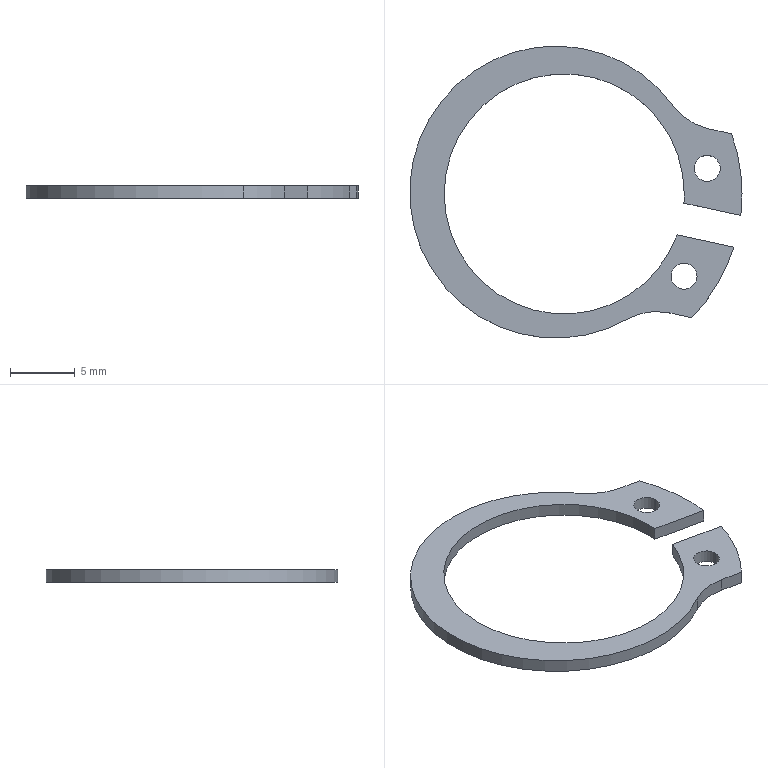Part | SolidWorks | features BaseBody 1 | 1 solid | 19 faces | box 25.605 x 22.5 x 1 mm | volume 159.858 mm3 | cylinder 13 | plane 6 | commonest cylinder face diameters 2 x4 18.5 x3 27.4 x3 9 x2 22.5 x1
STEP:
#1=CARTESIAN_POINT('',(-11.273,1593.906,-381.));
#2=VERTEX_POINT('',#1);
#3=CARTESIAN_POINT('',(-9.273,1593.906,-381.));
#4=VERTEX_POINT('',#3);
#5=CARTESIAN_POINT('',(-10.273,1593.906,-381.));
#6=DIRECTION('',(0.,0.,1.));
#7=DIRECTION('',(1.,0.,0.));
#8=AXIS2_PLACEMENT_3D('',#5,#6,#7);
#9=CIRCLE('',#8,1.);
#10=EDGE_CURVE('',#2,#4,#9,.T.);
#11=ORIENTED_EDGE('',*,*,#10,.F.);
#12=CARTESIAN_POINT('',(-11.273,1593.906,-380.));
#13=VERTEX_POINT('',#12);
#14=CARTESIAN_POINT('',(-11.273,1593.906,-381.));
#15=DIRECTION('',(0.,0.,1.));
#16=VECTOR('',#15,1000.);
#17=LINE('',#14,#16);
#18=EDGE_CURVE('',#2,#13,#17,.T.);
#19=ORIENTED_EDGE('',*,*,#18,.T.);
#20=CARTESIAN_POINT('',(-9.273,1593.906,-380.));
#21=VERTEX_POINT('',#20);
#22=CARTESIAN_POINT('',(-10.273,1593.906,-380.));
#23=DIRECTION('',(0.,0.,-1.));
#24=DIRECTION('',(1.,0.,0.));
#25=AXIS2_PLACEMENT_3D('',#22,#23,#24);
#26=CIRCLE('',#25,1.);
#27=EDGE_CURVE('',#21,#13,#26,.T.);
#28=ORIENTED_EDGE('',*,*,#27,.F.);
#29=CARTESIAN_POINT('',(-9.273,1593.906,-381.));
#30=DIRECTION('',(0.,0.,1.));
#31=VECTOR('',#30,1000.);
#32=LINE('',#29,#31);
#33=EDGE_CURVE('',#4,#21,#32,.T.);
#34=ORIENTED_EDGE('',*,*,#33,.F.);
#35=EDGE_LOOP('',(#11,#19,#28,#34));
#36=FACE_OUTER_BOUND('',#35,.T.);
#37=CARTESIAN_POINT('',(-10.273,1593.906,-381.));
#38=DIRECTION('',(0.,0.,1.));
#39=DIRECTION('',(1.,0.,0.));
#40=AXIS2_PLACEMENT_3D('',#37,#38,#39);
#41=CYLINDRICAL_SURFACE('',#40,1.);
#42=ADVANCED_FACE('',(#36),#41,.F.);
#43=CARTESIAN_POINT('',(-13.066,1585.597,-381.));
#44=VERTEX_POINT('',#43);
#45=CARTESIAN_POINT('',(-11.066,1585.597,-381.));
#46=VERTEX_POINT('',#45);
#47=CARTESIAN_POINT('',(-12.066,1585.597,-381.));
#48=DIRECTION('',(0.,0.,1.));
#49=DIRECTION('',(1.,0.,0.));
#50=AXIS2_PLACEMENT_3D('',#47,#48,#49);
#51=CIRCLE('',#50,1.);
#52=EDGE_CURVE('',#44,#46,#51,.T.);
#53=ORIENTED_EDGE('',*,*,#52,.F.);
#54=CARTESIAN_POINT('',(-13.066,1585.597,-380.));
#55=VERTEX_POINT('',#54);
#56=CARTESIAN_POINT('',(-13.066,1585.597,-381.));
#57=DIRECTION('',(0.,0.,1.));
#58=VECTOR('',#57,1000.);
#59=LINE('',#56,#58);
#60=EDGE_CURVE('',#44,#55,#59,.T.);
#61=ORIENTED_EDGE('',*,*,#60,.T.);
#62=CARTESIAN_POINT('',(-11.066,1585.597,-380.));
#63=VERTEX_POINT('',#62);
#64=CARTESIAN_POINT('',(-12.066,1585.597,-380.));
#65=DIRECTION('',(0.,0.,-1.));
#66=DIRECTION('',(1.,0.,0.));
#67=AXIS2_PLACEMENT_3D('',#64,#65,#66);
#68=CIRCLE('',#67,1.);
#69=EDGE_CURVE('',#63,#55,#68,.T.);
#70=ORIENTED_EDGE('',*,*,#69,.F.);
#71=CARTESIAN_POINT('',(-11.066,1585.597,-381.));
#72=DIRECTION('',(0.,0.,1.));
#73=VECTOR('',#72,1000.);
#74=LINE('',#71,#73);
#75=EDGE_CURVE('',#46,#63,#74,.T.);
#76=ORIENTED_EDGE('',*,*,#75,.F.);
#77=EDGE_LOOP('',(#53,#61,#70,#76));
#78=FACE_OUTER_BOUND('',#77,.T.);
#79=CARTESIAN_POINT('',(-12.066,1585.597,-381.));
#80=DIRECTION('',(0.,0.,1.));
#81=DIRECTION('',(1.,0.,0.));
#82=AXIS2_PLACEMENT_3D('',#79,#80,#81);
#83=CYLINDRICAL_SURFACE('',#82,1.);
#84=ADVANCED_FACE('',(#78),#83,.F.);
#85=CARTESIAN_POINT('',(-7.699,1590.281,-381.));
#86=VERTEX_POINT('',#85);
#87=CARTESIAN_POINT('',(-7.599,1591.937,-381.));
#88=VERTEX_POINT('',#87);
#89=CARTESIAN_POINT('',(-21.299,1591.937,-381.));
#90=DIRECTION('',(0.,0.,1.));
#91=DIRECTION('',(1.,0.,0.));
#92=AXIS2_PLACEMENT_3D('',#89,#90,#91);
#93=CIRCLE('',#92,13.7);
#94=EDGE_CURVE('',#86,#88,#93,.T.);
#95=ORIENTED_EDGE('',*,*,#94,.T.);
#96=CARTESIAN_POINT('',(-7.599,1591.937,-380.));
#97=VERTEX_POINT('',#96);
#98=CARTESIAN_POINT('',(-7.599,1591.937,-381.));
#99=DIRECTION('',(0.,0.,1.));
#100=VECTOR('',#99,1000.);
#101=LINE('',#98,#100);
#102=EDGE_CURVE('',#88,#97,#101,.T.);
#103=ORIENTED_EDGE('',*,*,#102,.T.);
#104=CARTESIAN_POINT('',(-7.699,1590.281,-380.));
#105=VERTEX_POINT('',#104);
#106=CARTESIAN_POINT('',(-21.299,1591.937,-380.));
#107=DIRECTION('',(0.,0.,1.));
#108=DIRECTION('',(1.,0.,0.));
#109=AXIS2_PLACEMENT_3D('',#106,#107,#108);
#110=CIRCLE('',#109,13.7);
#111=EDGE_CURVE('',#105,#97,#110,.T.);
#112=ORIENTED_EDGE('',*,*,#111,.F.);
#113=CARTESIAN_POINT('',(-7.699,1590.281,-381.));
#114=DIRECTION('',(0.,0.,-1.));
#115=VECTOR('',#114,1000.);
#116=LINE('',#113,#115);
#117=EDGE_CURVE('',#105,#86,#116,.T.);
#118=ORIENTED_EDGE('',*,*,#117,.T.);
#119=EDGE_LOOP('',(#95,#103,#112,#118));
#120=FACE_OUTER_BOUND('',#119,.T.);
#121=CARTESIAN_POINT('',(-21.299,1591.937,-381.));
#122=DIRECTION('',(0.,0.,1.));
#123=DIRECTION('',(1.,0.,0.));
#124=AXIS2_PLACEMENT_3D('',#121,#122,#123);
#125=CYLINDRICAL_SURFACE('',#124,13.7);
#126=ADVANCED_FACE('',(#120),#125,.T.);
#127=CARTESIAN_POINT('',(-30.549,1591.937,-381.));
#128=VERTEX_POINT('',#127);
#129=CARTESIAN_POINT('',(-12.603,1588.782,-381.));
#130=VERTEX_POINT('',#129);
#131=CARTESIAN_POINT('',(-21.299,1591.937,-381.));
#132=DIRECTION('',(0.,0.,1.));
#133=DIRECTION('',(1.,0.,0.));
#134=AXIS2_PLACEMENT_3D('',#131,#132,#133);
#135=CIRCLE('',#134,9.25);
#136=EDGE_CURVE('',#128,#130,#135,.T.);
#137=ORIENTED_EDGE('',*,*,#136,.F.);
#138=CARTESIAN_POINT('',(-30.549,1591.937,-380.));
#139=VERTEX_POINT('',#138);
#140=CARTESIAN_POINT('',(-30.549,1591.937,-381.));
#141=DIRECTION('',(0.,0.,1.));
#142=VECTOR('',#141,1000.);
#143=LINE('',#140,#142);
#144=EDGE_CURVE('',#128,#139,#143,.T.);
#145=ORIENTED_EDGE('',*,*,#144,.T.);
#146=CARTESIAN_POINT('',(-12.603,1588.782,-380.));
#147=VERTEX_POINT('',#146);
#148=CARTESIAN_POINT('',(-21.299,1591.937,-380.));
#149=DIRECTION('',(0.,0.,-1.));
#150=DIRECTION('',(1.,0.,0.));
#151=AXIS2_PLACEMENT_3D('',#148,#149,#150);
#152=CIRCLE('',#151,9.25);
#153=EDGE_CURVE('',#147,#139,#152,.T.);
#154=ORIENTED_EDGE('',*,*,#153,.F.);
#155=CARTESIAN_POINT('',(-12.603,1588.782,-381.));
#156=DIRECTION('',(0.,0.,1.));
#157=VECTOR('',#156,1000.);
#158=LINE('',#155,#157);
#159=EDGE_CURVE('',#130,#147,#158,.T.);
#160=ORIENTED_EDGE('',*,*,#159,.F.);
#161=EDGE_LOOP('',(#137,#145,#154,#160));
#162=FACE_OUTER_BOUND('',#161,.T.);
#163=CARTESIAN_POINT('',(-21.299,1591.937,-381.));
#164=DIRECTION('',(0.,0.,1.));
#165=DIRECTION('',(1.,0.,0.));
#166=AXIS2_PLACEMENT_3D('',#163,#164,#165);
#167=CYLINDRICAL_SURFACE('',#166,9.25);
#168=ADVANCED_FACE('',(#162),#167,.F.);
#169=ORIENTED_EDGE('',*,*,#144,.F.);
#170=CARTESIAN_POINT('',(-12.049,1591.937,-381.));
#171=VERTEX_POINT('',#170);
#172=CARTESIAN_POINT('',(-21.299,1591.937,-381.));
#173=DIRECTION('',(0.,0.,1.));
#174=DIRECTION('',(1.,0.,0.));
#175=AXIS2_PLACEMENT_3D('',#172,#173,#174);
#176=CIRCLE('',#175,9.25);
#177=EDGE_CURVE('',#171,#128,#176,.T.);
#178=ORIENTED_EDGE('',*,*,#177,.F.);
#179=CARTESIAN_POINT('',(-12.049,1591.937,-380.));
#180=VERTEX_POINT('',#179);
#181=CARTESIAN_POINT('',(-12.049,1591.937,-381.));
#182=DIRECTION('',(0.,0.,1.));
#183=VECTOR('',#182,1000.);
#184=LINE('',#181,#183);
#185=EDGE_CURVE('',#171,#180,#184,.T.);
#186=ORIENTED_EDGE('',*,*,#185,.T.);
#187=CARTESIAN_POINT('',(-21.299,1591.937,-380.));
#188=DIRECTION('',(0.,0.,-1.));
#189=DIRECTION('',(1.,0.,0.));
#190=AXIS2_PLACEMENT_3D('',#187,#188,#189);
#191=CIRCLE('',#190,9.25);
#192=EDGE_CURVE('',#139,#180,#191,.T.);
#193=ORIENTED_EDGE('',*,*,#192,.F.);
#194=EDGE_LOOP('',(#169,#178,#186,#193));
#195=FACE_OUTER_BOUND('',#194,.T.);
#196=CARTESIAN_POINT('',(-21.299,1591.937,-381.));
#197=DIRECTION('',(0.,0.,1.));
#198=DIRECTION('',(1.,0.,0.));
#199=AXIS2_PLACEMENT_3D('',#196,#197,#198);
#200=CYLINDRICAL_SURFACE('',#199,9.25);
#201=ADVANCED_FACE('',(#195),#200,.F.);
#202=ORIENTED_EDGE('',*,*,#27,.T.);
#203=CARTESIAN_POINT('',(-10.273,1593.906,-380.));
#204=DIRECTION('',(0.,0.,-1.));
#205=DIRECTION('',(1.,0.,0.));
#206=AXIS2_PLACEMENT_3D('',#203,#204,#205);
#207=CIRCLE('',#206,1.);
#208=EDGE_CURVE('',#13,#21,#207,.T.);
#209=ORIENTED_EDGE('',*,*,#208,.T.);
#210=EDGE_LOOP('',(#202,#209));
#211=FACE_BOUND('',#210,.T.);
#212=ORIENTED_EDGE('',*,*,#69,.T.);
#213=CARTESIAN_POINT('',(-12.066,1585.597,-380.));
#214=DIRECTION('',(0.,0.,-1.));
#215=DIRECTION('',(1.,0.,0.));
#216=AXIS2_PLACEMENT_3D('',#213,#214,#215);
#217=CIRCLE('',#216,1.);
#218=EDGE_CURVE('',#55,#63,#217,.T.);
#219=ORIENTED_EDGE('',*,*,#218,.T.);
#220=EDGE_LOOP('',(#212,#219));
#221=FACE_BOUND('',#220,.T.);
#222=ORIENTED_EDGE('',*,*,#111,.T.);
#223=CARTESIAN_POINT('',(-8.406,1596.572,-380.));
#224=VERTEX_POINT('',#223);
#225=CARTESIAN_POINT('',(-21.299,1591.937,-380.));
#226=DIRECTION('',(0.,0.,1.));
#227=DIRECTION('',(1.,0.,0.));
#228=AXIS2_PLACEMENT_3D('',#225,#226,#227);
#229=CIRCLE('',#228,13.7);
#230=EDGE_CURVE('',#97,#224,#229,.T.);
#231=ORIENTED_EDGE('',*,*,#230,.T.);
#232=CARTESIAN_POINT('',(-10.172,1596.953,-380.));
#233=VERTEX_POINT('',#232);
#234=CARTESIAN_POINT('',(-8.406,1596.572,-380.));
#235=DIRECTION('',(-0.9775,0.2109,0.));
#236=VECTOR('',#235,1000.);
#237=LINE('',#234,#236);
#238=EDGE_CURVE('',#224,#233,#237,.T.);
#239=ORIENTED_EDGE('',*,*,#238,.T.);
#240=CARTESIAN_POINT('',(-12.86,1598.702,-380.));
#241=VERTEX_POINT('',#240);
#242=CARTESIAN_POINT('',(-9.223,1601.352,-380.));
#243=DIRECTION('',(0.,0.,-1.));
#244=DIRECTION('',(1.,0.,0.));
#245=AXIS2_PLACEMENT_3D('',#242,#243,#244);
#246=CIRCLE('',#245,4.5);
#247=EDGE_CURVE('',#233,#241,#246,.T.);
#248=ORIENTED_EDGE('',*,*,#247,.T.);
#249=CARTESIAN_POINT('',(-16.401,1582.294,-380.));
#250=VERTEX_POINT('',#249);
#251=CARTESIAN_POINT('',(-21.953,1592.079,-380.));
#252=DIRECTION('',(0.,0.,1.));
#253=DIRECTION('',(1.,0.,0.));
#254=AXIS2_PLACEMENT_3D('',#251,#252,#253);
#255=CIRCLE('',#254,11.25);
#256=EDGE_CURVE('',#241,#250,#255,.T.);
#257=ORIENTED_EDGE('',*,*,#256,.T.);
#258=CARTESIAN_POINT('',(-13.231,1582.779,-380.));
#259=VERTEX_POINT('',#258);
#260=CARTESIAN_POINT('',(-14.18,1578.381,-380.));
#261=DIRECTION('',(0.,0.,-1.));
#262=DIRECTION('',(1.,0.,0.));
#263=AXIS2_PLACEMENT_3D('',#260,#261,#262);
#264=CIRCLE('',#263,4.5);
#265=EDGE_CURVE('',#250,#259,#264,.T.);
#266=ORIENTED_EDGE('',*,*,#265,.T.);
#267=CARTESIAN_POINT('',(-11.465,1582.398,-380.));
#268=VERTEX_POINT('',#267);
#269=CARTESIAN_POINT('',(-13.231,1582.779,-380.));
#270=DIRECTION('',(0.9775,-0.2109,0.));
#271=VECTOR('',#270,1000.);
#272=LINE('',#269,#271);
#273=EDGE_CURVE('',#259,#268,#272,.T.);
#274=ORIENTED_EDGE('',*,*,#273,.T.);
#275=CARTESIAN_POINT('',(-8.226,1587.838,-380.));
#276=VERTEX_POINT('',#275);
#277=CARTESIAN_POINT('',(-21.299,1591.937,-380.));
#278=DIRECTION('',(0.,0.,1.));
#279=DIRECTION('',(1.,0.,0.));
#280=AXIS2_PLACEMENT_3D('',#277,#278,#279);
#281=CIRCLE('',#280,13.7);
#282=EDGE_CURVE('',#268,#276,#281,.T.);
#283=ORIENTED_EDGE('',*,*,#282,.T.);
#284=CARTESIAN_POINT('',(-8.226,1587.838,-380.));
#285=DIRECTION('',(-0.9775,0.2109,0.));
#286=VECTOR('',#285,1000.);
#287=LINE('',#284,#286);
#288=EDGE_CURVE('',#276,#147,#287,.T.);
#289=ORIENTED_EDGE('',*,*,#288,.T.);
#290=ORIENTED_EDGE('',*,*,#153,.T.);
#291=ORIENTED_EDGE('',*,*,#192,.T.);
#292=CARTESIAN_POINT('',(-12.076,1591.226,-380.));
#293=VERTEX_POINT('',#292);
#294=CARTESIAN_POINT('',(-21.299,1591.937,-380.));
#295=DIRECTION('',(0.,0.,-1.));
#296=DIRECTION('',(1.,0.,0.));
#297=AXIS2_PLACEMENT_3D('',#294,#295,#296);
#298=CIRCLE('',#297,9.25);
#299=EDGE_CURVE('',#180,#293,#298,.T.);
#300=ORIENTED_EDGE('',*,*,#299,.T.);
#301=CARTESIAN_POINT('',(-12.076,1591.226,-380.));
#302=DIRECTION('',(0.9775,-0.2109,0.));
#303=VECTOR('',#302,1000.);
#304=LINE('',#301,#303);
#305=EDGE_CURVE('',#293,#105,#304,.T.);
#306=ORIENTED_EDGE('',*,*,#305,.T.);
#307=EDGE_LOOP('',(#222,#231,#239,#248,#257,#266,#274,#283,#289,#290,#291,#300,#306));
#308=FACE_OUTER_BOUND('',#307,.T.);
#309=CARTESIAN_POINT('',(-21.953,1592.079,-380.));
#310=DIRECTION('',(0.,0.,1.));
#311=DIRECTION('',(1.,0.,0.));
#312=AXIS2_PLACEMENT_3D('',#309,#310,#311);
#313=PLANE('',#312);
#314=ADVANCED_FACE('',(#211,#221,#308),#313,.T.);
#315=ORIENTED_EDGE('',*,*,#18,.F.);
#316=CARTESIAN_POINT('',(-10.273,1593.906,-381.));
#317=DIRECTION('',(0.,0.,1.));
#318=DIRECTION('',(1.,0.,0.));
#319=AXIS2_PLACEMENT_3D('',#316,#317,#318);
#320=CIRCLE('',#319,1.);
#321=EDGE_CURVE('',#4,#2,#320,.T.);
#322=ORIENTED_EDGE('',*,*,#321,.F.);
#323=ORIENTED_EDGE('',*,*,#33,.T.);
#324=ORIENTED_EDGE('',*,*,#208,.F.);
#325=EDGE_LOOP('',(#315,#322,#323,#324));
#326=FACE_OUTER_BOUND('',#325,.T.);
#327=CARTESIAN_POINT('',(-10.273,1593.906,-381.));
#328=DIRECTION('',(0.,0.,1.));
#329=DIRECTION('',(1.,0.,0.));
#330=AXIS2_PLACEMENT_3D('',#327,#328,#329);
#331=CYLINDRICAL_SURFACE('',#330,1.);
#332=ADVANCED_FACE('',(#326),#331,.F.);
#333=ORIENTED_EDGE('',*,*,#60,.F.);
#334=CARTESIAN_POINT('',(-12.066,1585.597,-381.));
#335=DIRECTION('',(0.,0.,1.));
#336=DIRECTION('',(1.,0.,0.));
#337=AXIS2_PLACEMENT_3D('',#334,#335,#336);
#338=CIRCLE('',#337,1.);
#339=EDGE_CURVE('',#46,#44,#338,.T.);
#340=ORIENTED_EDGE('',*,*,#339,.F.);
#341=ORIENTED_EDGE('',*,*,#75,.T.);
#342=ORIENTED_EDGE('',*,*,#218,.F.);
#343=EDGE_LOOP('',(#333,#340,#341,#342));
#344=FACE_OUTER_BOUND('',#343,.T.);
#345=CARTESIAN_POINT('',(-12.066,1585.597,-381.));
#346=DIRECTION('',(0.,0.,1.));
#347=DIRECTION('',(1.,0.,0.));
#348=AXIS2_PLACEMENT_3D('',#345,#346,#347);
#349=CYLINDRICAL_SURFACE('',#348,1.);
#350=ADVANCED_FACE('',(#344),#349,.F.);
#351=CARTESIAN_POINT('',(-8.406,1596.572,-381.));
#352=VERTEX_POINT('',#351);
#353=CARTESIAN_POINT('',(-8.406,1596.572,-381.));
#354=DIRECTION('',(0.,0.,-1.));
#355=VECTOR('',#354,1000.);
#356=LINE('',#353,#355);
#357=EDGE_CURVE('',#224,#352,#356,.T.);
#358=ORIENTED_EDGE('',*,*,#357,.T.);
#359=CARTESIAN_POINT('',(-10.172,1596.953,-381.));
#360=VERTEX_POINT('',#359);
#361=CARTESIAN_POINT('',(-12.015,1597.351,-381.));
#362=DIRECTION('',(-0.9775,0.2109,0.));
#363=VECTOR('',#362,1000.);
#364=LINE('',#361,#363);
#365=EDGE_CURVE('',#352,#360,#364,.T.);
#366=ORIENTED_EDGE('',*,*,#365,.T.);
#367=CARTESIAN_POINT('',(-10.172,1596.953,-381.));
#368=DIRECTION('',(0.,0.,1.));
#369=VECTOR('',#368,1000.);
#370=LINE('',#367,#369);
#371=EDGE_CURVE('',#360,#233,#370,.T.);
#372=ORIENTED_EDGE('',*,*,#371,.T.);
#373=ORIENTED_EDGE('',*,*,#238,.F.);
#374=EDGE_LOOP('',(#358,#366,#372,#373));
#375=FACE_OUTER_BOUND('',#374,.T.);
#376=CARTESIAN_POINT('',(-12.015,1597.351,-381.));
#377=DIRECTION('',(0.2109,0.9775,0.));
#378=DIRECTION('',(-0.9775,0.2109,0.));
#379=AXIS2_PLACEMENT_3D('',#376,#377,#378);
#380=PLANE('',#379);
#381=ADVANCED_FACE('',(#375),#380,.T.);
#382=ORIENTED_EDGE('',*,*,#102,.F.);
#383=CARTESIAN_POINT('',(-21.299,1591.937,-381.));
#384=DIRECTION('',(0.,0.,1.));
#385=DIRECTION('',(1.,0.,0.));
#386=AXIS2_PLACEMENT_3D('',#383,#384,#385);
#387=CIRCLE('',#386,13.7);
#388=EDGE_CURVE('',#88,#352,#387,.T.);
#389=ORIENTED_EDGE('',*,*,#388,.T.);
#390=ORIENTED_EDGE('',*,*,#357,.F.);
#391=ORIENTED_EDGE('',*,*,#230,.F.);
#392=EDGE_LOOP('',(#382,#389,#390,#391));
#393=FACE_OUTER_BOUND('',#392,.T.);
#394=CARTESIAN_POINT('',(-21.299,1591.937,-381.));
#395=DIRECTION('',(0.,0.,1.));
#396=DIRECTION('',(1.,0.,0.));
#397=AXIS2_PLACEMENT_3D('',#394,#395,#396);
#398=CYLINDRICAL_SURFACE('',#397,13.7);
#399=ADVANCED_FACE('',(#393),#398,.T.);
#400=ORIENTED_EDGE('',*,*,#117,.F.);
#401=ORIENTED_EDGE('',*,*,#305,.F.);
#402=CARTESIAN_POINT('',(-12.076,1591.226,-381.));
#403=VERTEX_POINT('',#402);
#404=CARTESIAN_POINT('',(-12.076,1591.226,-381.));
#405=DIRECTION('',(0.,0.,-1.));
#406=VECTOR('',#405,1000.);
#407=LINE('',#404,#406);
#408=EDGE_CURVE('',#293,#403,#407,.T.);
#409=ORIENTED_EDGE('',*,*,#408,.T.);
#410=CARTESIAN_POINT('',(-7.699,1590.281,-381.));
#411=DIRECTION('',(0.9775,-0.2109,0.));
#412=VECTOR('',#411,1000.);
#413=LINE('',#410,#412);
#414=EDGE_CURVE('',#403,#86,#413,.T.);
#415=ORIENTED_EDGE('',*,*,#414,.T.);
#416=EDGE_LOOP('',(#400,#401,#409,#415));
#417=FACE_OUTER_BOUND('',#416,.T.);
#418=CARTESIAN_POINT('',(-7.699,1590.281,-381.));
#419=DIRECTION('',(-0.2109,-0.9775,0.));
#420=DIRECTION('',(0.9775,-0.2109,0.));
#421=AXIS2_PLACEMENT_3D('',#418,#419,#420);
#422=PLANE('',#421);
#423=ADVANCED_FACE('',(#417),#422,.T.);
#424=ORIENTED_EDGE('',*,*,#185,.F.);
#425=CARTESIAN_POINT('',(-21.299,1591.937,-381.));
#426=DIRECTION('',(0.,0.,1.));
#427=DIRECTION('',(1.,0.,0.));
#428=AXIS2_PLACEMENT_3D('',#425,#426,#427);
#429=CIRCLE('',#428,9.25);
#430=EDGE_CURVE('',#403,#171,#429,.T.);
#431=ORIENTED_EDGE('',*,*,#430,.F.);
#432=ORIENTED_EDGE('',*,*,#408,.F.);
#433=ORIENTED_EDGE('',*,*,#299,.F.);
#434=EDGE_LOOP('',(#424,#431,#432,#433));
#435=FACE_OUTER_BOUND('',#434,.T.);
#436=CARTESIAN_POINT('',(-21.299,1591.937,-381.));
#437=DIRECTION('',(0.,0.,1.));
#438=DIRECTION('',(1.,0.,0.));
#439=AXIS2_PLACEMENT_3D('',#436,#437,#438);
#440=CYLINDRICAL_SURFACE('',#439,9.25);
#441=ADVANCED_FACE('',(#435),#440,.F.);
#442=ORIENTED_EDGE('',*,*,#159,.T.);
#443=ORIENTED_EDGE('',*,*,#288,.F.);
#444=CARTESIAN_POINT('',(-8.226,1587.838,-381.));
#445=VERTEX_POINT('',#444);
#446=CARTESIAN_POINT('',(-8.226,1587.838,-381.));
#447=DIRECTION('',(0.,0.,-1.));
#448=VECTOR('',#447,1000.);
#449=LINE('',#446,#448);
#450=EDGE_CURVE('',#276,#445,#449,.T.);
#451=ORIENTED_EDGE('',*,*,#450,.T.);
#452=CARTESIAN_POINT('',(-8.226,1587.838,-381.));
#453=DIRECTION('',(-0.9775,0.2109,0.));
#454=VECTOR('',#453,1000.);
#455=LINE('',#452,#454);
#456=EDGE_CURVE('',#445,#130,#455,.T.);
#457=ORIENTED_EDGE('',*,*,#456,.T.);
#458=EDGE_LOOP('',(#442,#443,#451,#457));
#459=FACE_OUTER_BOUND('',#458,.T.);
#460=CARTESIAN_POINT('',(-8.226,1587.838,-381.));
#461=DIRECTION('',(0.2109,0.9775,0.));
#462=DIRECTION('',(-0.9775,0.2109,0.));
#463=AXIS2_PLACEMENT_3D('',#460,#461,#462);
#464=PLANE('',#463);
#465=ADVANCED_FACE('',(#459),#464,.T.);
#466=ORIENTED_EDGE('',*,*,#450,.F.);
#467=ORIENTED_EDGE('',*,*,#282,.F.);
#468=CARTESIAN_POINT('',(-11.465,1582.398,-381.));
#469=VERTEX_POINT('',#468);
#470=CARTESIAN_POINT('',(-11.465,1582.398,-381.));
#471=DIRECTION('',(0.,0.,-1.));
#472=VECTOR('',#471,1000.);
#473=LINE('',#470,#472);
#474=EDGE_CURVE('',#268,#469,#473,.T.);
#475=ORIENTED_EDGE('',*,*,#474,.T.);
#476=CARTESIAN_POINT('',(-21.299,1591.937,-381.));
#477=DIRECTION('',(0.,0.,1.));
#478=DIRECTION('',(1.,0.,0.));
#479=AXIS2_PLACEMENT_3D('',#476,#477,#478);
#480=CIRCLE('',#479,13.7);
#481=EDGE_CURVE('',#469,#445,#480,.T.);
#482=ORIENTED_EDGE('',*,*,#481,.T.);
#483=EDGE_LOOP('',(#466,#467,#475,#482));
#484=FACE_OUTER_BOUND('',#483,.T.);
#485=CARTESIAN_POINT('',(-21.299,1591.937,-381.));
#486=DIRECTION('',(0.,0.,1.));
#487=DIRECTION('',(1.,0.,0.));
#488=AXIS2_PLACEMENT_3D('',#485,#486,#487);
#489=CYLINDRICAL_SURFACE('',#488,13.7);
#490=ADVANCED_FACE('',(#484),#489,.T.);
#491=ORIENTED_EDGE('',*,*,#474,.F.);
#492=ORIENTED_EDGE('',*,*,#273,.F.);
#493=CARTESIAN_POINT('',(-13.231,1582.779,-381.));
#494=VERTEX_POINT('',#493);
#495=CARTESIAN_POINT('',(-13.231,1582.779,-381.));
#496=DIRECTION('',(0.,0.,-1.));
#497=VECTOR('',#496,1000.);
#498=LINE('',#495,#497);
#499=EDGE_CURVE('',#259,#494,#498,.T.);
#500=ORIENTED_EDGE('',*,*,#499,.T.);
#501=CARTESIAN_POINT('',(-15.074,1583.177,-381.));
#502=DIRECTION('',(0.9775,-0.2109,0.));
#503=VECTOR('',#502,1000.);
#504=LINE('',#501,#503);
#505=EDGE_CURVE('',#494,#469,#504,.T.);
#506=ORIENTED_EDGE('',*,*,#505,.T.);
#507=EDGE_LOOP('',(#491,#492,#500,#506));
#508=FACE_OUTER_BOUND('',#507,.T.);
#509=CARTESIAN_POINT('',(-15.074,1583.177,-381.));
#510=DIRECTION('',(-0.2109,-0.9775,0.));
#511=DIRECTION('',(0.9775,-0.2109,0.));
#512=AXIS2_PLACEMENT_3D('',#509,#510,#511);
#513=PLANE('',#512);
#514=ADVANCED_FACE('',(#508),#513,.T.);
#515=ORIENTED_EDGE('',*,*,#265,.F.);
#516=CARTESIAN_POINT('',(-16.401,1582.294,-381.));
#517=VERTEX_POINT('',#516);
#518=CARTESIAN_POINT('',(-16.401,1582.294,-381.));
#519=DIRECTION('',(0.,0.,1.));
#520=VECTOR('',#519,1000.);
#521=LINE('',#518,#520);
#522=EDGE_CURVE('',#517,#250,#521,.T.);
#523=ORIENTED_EDGE('',*,*,#522,.F.);
#524=CARTESIAN_POINT('',(-14.18,1578.381,-381.));
#525=DIRECTION('',(0.,0.,1.));
#526=DIRECTION('',(1.,0.,0.));
#527=AXIS2_PLACEMENT_3D('',#524,#525,#526);
#528=CIRCLE('',#527,4.5);
#529=EDGE_CURVE('',#494,#517,#528,.T.);
#530=ORIENTED_EDGE('',*,*,#529,.F.);
#531=ORIENTED_EDGE('',*,*,#499,.F.);
#532=EDGE_LOOP('',(#515,#523,#530,#531));
#533=FACE_OUTER_BOUND('',#532,.T.);
#534=CARTESIAN_POINT('',(-14.18,1578.381,-381.));
#535=DIRECTION('',(0.,0.,1.));
#536=DIRECTION('',(1.,0.,0.));
#537=AXIS2_PLACEMENT_3D('',#534,#535,#536);
#538=CYLINDRICAL_SURFACE('',#537,4.5);
#539=ADVANCED_FACE('',(#533),#538,.F.);
#540=CARTESIAN_POINT('',(-12.86,1598.702,-381.));
#541=VERTEX_POINT('',#540);
#542=CARTESIAN_POINT('',(-12.86,1598.702,-381.));
#543=DIRECTION('',(0.,0.,-1.));
#544=VECTOR('',#543,1000.);
#545=LINE('',#542,#544);
#546=EDGE_CURVE('',#241,#541,#545,.T.);
#547=ORIENTED_EDGE('',*,*,#546,.T.);
#548=CARTESIAN_POINT('',(-21.953,1592.079,-381.));
#549=DIRECTION('',(0.,0.,1.));
#550=DIRECTION('',(1.,0.,0.));
#551=AXIS2_PLACEMENT_3D('',#548,#549,#550);
#552=CIRCLE('',#551,11.25);
#553=EDGE_CURVE('',#541,#517,#552,.T.);
#554=ORIENTED_EDGE('',*,*,#553,.T.);
#555=ORIENTED_EDGE('',*,*,#522,.T.);
#556=ORIENTED_EDGE('',*,*,#256,.F.);
#557=EDGE_LOOP('',(#547,#554,#555,#556));
#558=FACE_OUTER_BOUND('',#557,.T.);
#559=CARTESIAN_POINT('',(-21.953,1592.079,-381.));
#560=DIRECTION('',(0.,0.,1.));
#561=DIRECTION('',(1.,0.,0.));
#562=AXIS2_PLACEMENT_3D('',#559,#560,#561);
#563=CYLINDRICAL_SURFACE('',#562,11.25);
#564=ADVANCED_FACE('',(#558),#563,.T.);
#565=ORIENTED_EDGE('',*,*,#247,.F.);
#566=ORIENTED_EDGE('',*,*,#371,.F.);
#567=CARTESIAN_POINT('',(-9.223,1601.352,-381.));
#568=DIRECTION('',(0.,0.,1.));
#569=DIRECTION('',(1.,0.,0.));
#570=AXIS2_PLACEMENT_3D('',#567,#568,#569);
#571=CIRCLE('',#570,4.5);
#572=EDGE_CURVE('',#541,#360,#571,.T.);
#573=ORIENTED_EDGE('',*,*,#572,.F.);
#574=ORIENTED_EDGE('',*,*,#546,.F.);
#575=EDGE_LOOP('',(#565,#566,#573,#574));
#576=FACE_OUTER_BOUND('',#575,.T.);
#577=CARTESIAN_POINT('',(-9.223,1601.352,-381.));
#578=DIRECTION('',(0.,0.,1.));
#579=DIRECTION('',(1.,0.,0.));
#580=AXIS2_PLACEMENT_3D('',#577,#578,#579);
#581=CYLINDRICAL_SURFACE('',#580,4.5);
#582=ADVANCED_FACE('',(#576),#581,.F.);
#583=ORIENTED_EDGE('',*,*,#321,.T.);
#584=ORIENTED_EDGE('',*,*,#10,.T.);
#585=EDGE_LOOP('',(#583,#584));
#586=FACE_BOUND('',#585,.T.);
#587=ORIENTED_EDGE('',*,*,#339,.T.);
#588=ORIENTED_EDGE('',*,*,#52,.T.);
#589=EDGE_LOOP('',(#587,#588));
#590=FACE_BOUND('',#589,.T.);
#591=ORIENTED_EDGE('',*,*,#365,.F.);
#592=ORIENTED_EDGE('',*,*,#388,.F.);
#593=ORIENTED_EDGE('',*,*,#94,.F.);
#594=ORIENTED_EDGE('',*,*,#414,.F.);
#595=ORIENTED_EDGE('',*,*,#430,.T.);
#596=ORIENTED_EDGE('',*,*,#177,.T.);
#597=ORIENTED_EDGE('',*,*,#136,.T.);
#598=ORIENTED_EDGE('',*,*,#456,.F.);
#599=ORIENTED_EDGE('',*,*,#481,.F.);
#600=ORIENTED_EDGE('',*,*,#505,.F.);
#601=ORIENTED_EDGE('',*,*,#529,.T.);
#602=ORIENTED_EDGE('',*,*,#553,.F.);
#603=ORIENTED_EDGE('',*,*,#572,.T.);
#604=EDGE_LOOP('',(#591,#592,#593,#594,#595,#596,#597,#598,#599,#600,#601,#602,#603));
#605=FACE_OUTER_BOUND('',#604,.T.);
#606=CARTESIAN_POINT('',(-21.953,1592.079,-381.));
#607=DIRECTION('',(0.,0.,1.));
#608=DIRECTION('',(1.,0.,0.));
#609=AXIS2_PLACEMENT_3D('',#606,#607,#608);
#610=PLANE('',#609);
#611=ADVANCED_FACE('',(#586,#590,#605),#610,.F.);
#612=CLOSED_SHELL('',(#42,#84,#126,#168,#201,#314,#332,#350,#381,#399,#423,#441,#465,#490,#514,#539,#564,#582,#611));
#613=MANIFOLD_SOLID_BREP('',#612);
#614=CARTESIAN_POINT('',(0.,0.,0.));
#615=DIRECTION('',(0.,0.,1.));
#616=DIRECTION('',(1.,0.,0.));
#617=AXIS2_PLACEMENT_3D('',#614,#615,#616);
#618=(LENGTH_UNIT()NAMED_UNIT(*)SI_UNIT(.MILLI.,.METRE.));
#619=UNCERTAINTY_MEASURE_WITH_UNIT(LENGTH_MEASURE(0.00001),#618,'','');
#620=(NAMED_UNIT(*)PLANE_ANGLE_UNIT()SI_UNIT($,.RADIAN.));
#621=(NAMED_UNIT(*)SI_UNIT($,.STERADIAN.)SOLID_ANGLE_UNIT());
#622=(GEOMETRIC_REPRESENTATION_CONTEXT(3)GLOBAL_UNCERTAINTY_ASSIGNED_CONTEXT((#619))GLOBAL_UNIT_ASSIGNED_CONTEXT((#618,#620,#621))REPRESENTATION_CONTEXT('',''));
#623=ADVANCED_BREP_SHAPE_REPRESENTATION('',(#613,#617),#622);